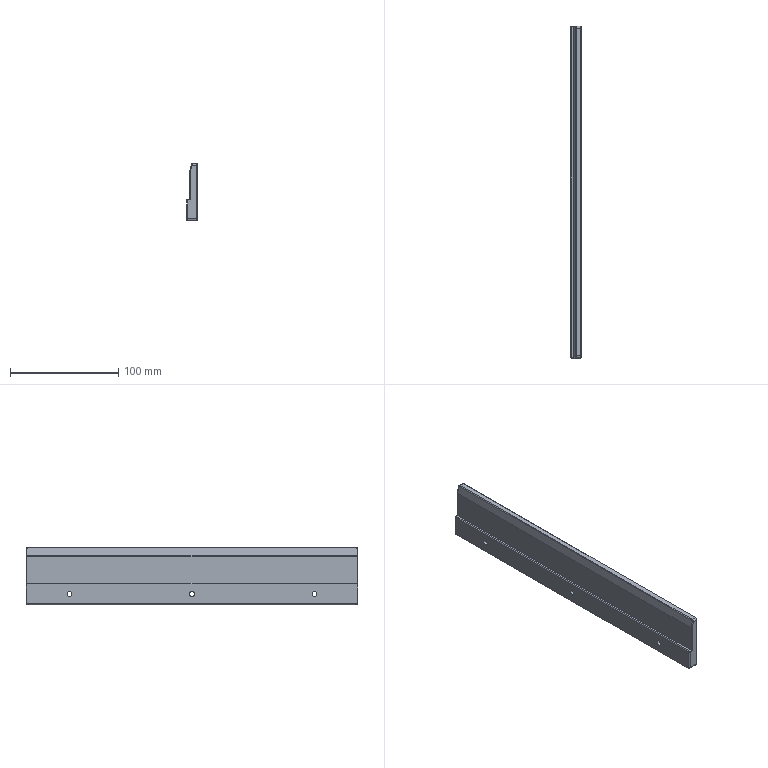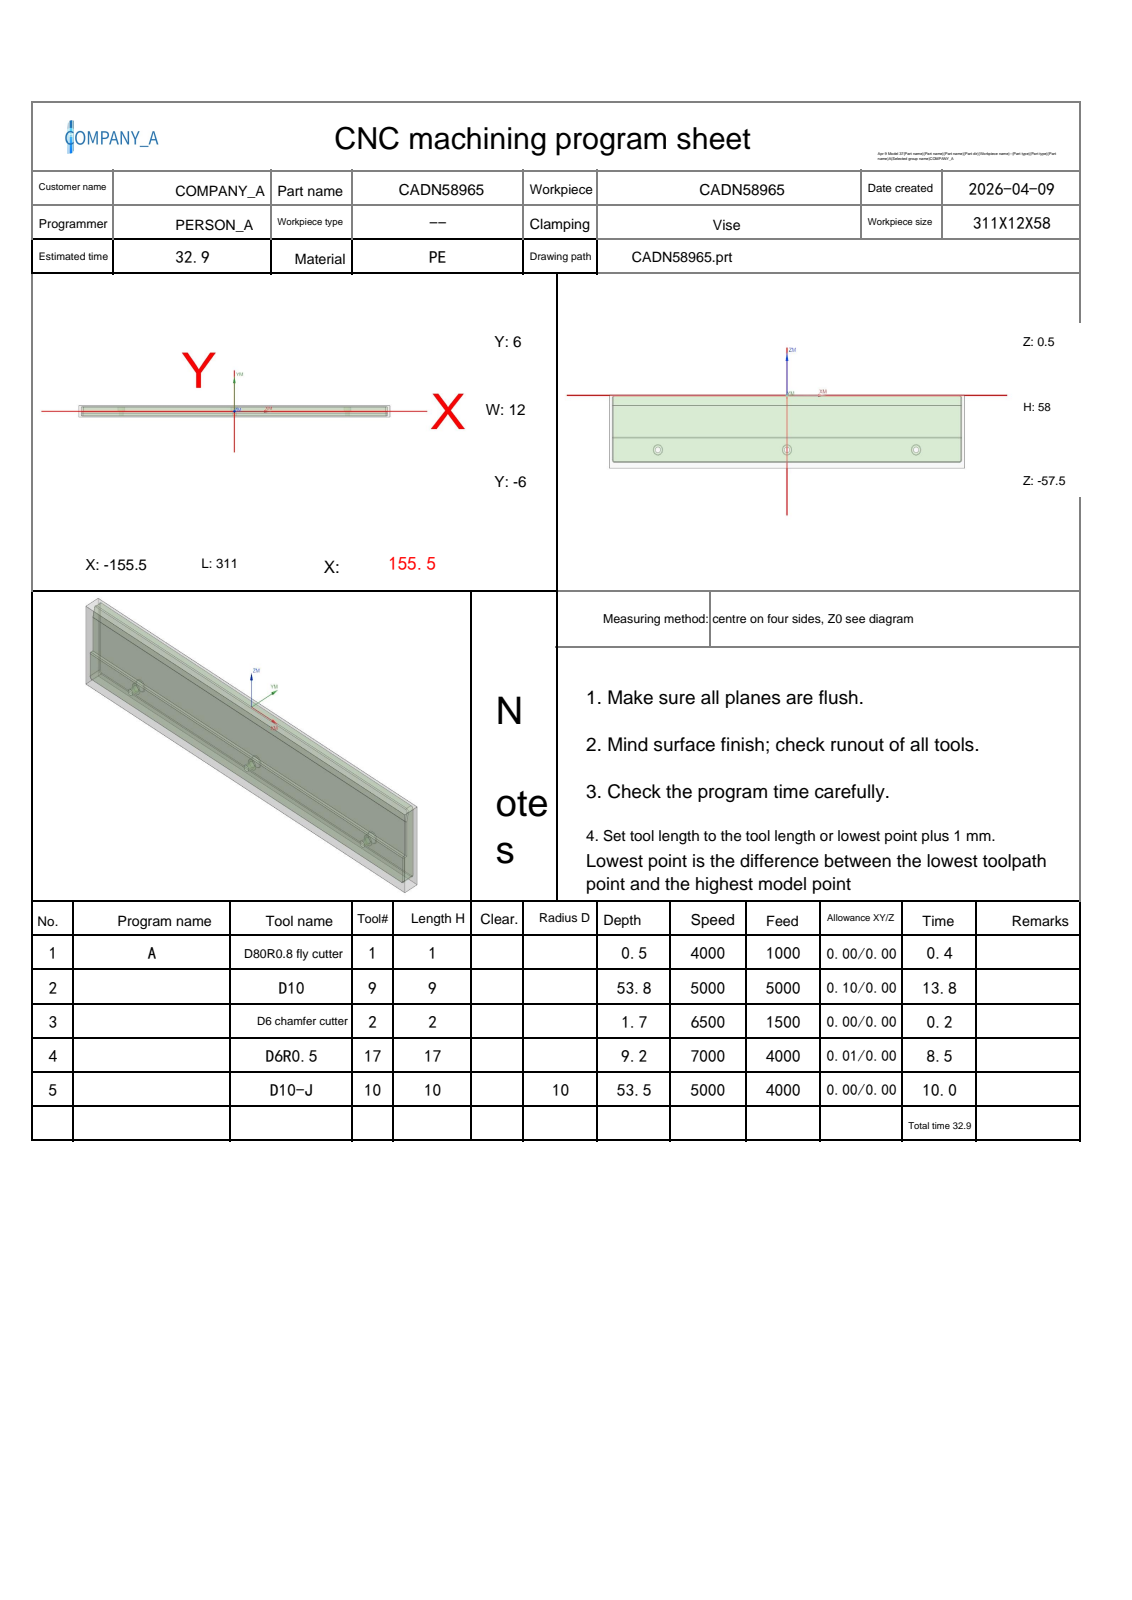NC program | NX | posted by the shop | part box 10 x 306 x 53 mm
Lines 1290 to 3098 of 3792, first 1630 of 1809 lines:
N4 T17 M06
(D6R0.5  D=6. R=0.5 H=17 ce=0.01 di=0.00)
G00 G90 G54 X148.205 Y10.104 M03 S7000
G43 H17 Z10.5
M08
Z.491
G01 Z-.009 F4000.
X148.307 Y8.501
G03 X149.804 Y7.096 I1.497 J.095
G01 X149.899 Y7.099
G02 X150.429 Y7.116 I.53 J-8.323
X151.333 Y7.067 I0.0 J-8.34
X153.721 Y4.5 I-.291 J-2.664
G01 Y.309
G02 X151.052 Y-2.343 I-2.743 J.091
G01 X149.898 Y-2.373
Y-2.418 Z-.015
Y-2.454 Z-.021
X151.047 Y-2.437
G03 X153.836 Y.283 I-.042 J2.833
G01 Y4.5
G03 X151.122 Y7.137 I-2.737 J-.102
G01 X149.9 Y7.147
Y7.179 Z-.03
Y7.2 Z-.038
G02 X150.426 Y7.214 I.526 J-9.546
X151.615 Y7.14 I0.0 J-9.56
X153.943 Y4.502 I-.331 J-2.638
G01 Y.281
G02 X151.111 Y-2.506 I-2.888 J.103
G01 X149.898 Y-2.53
Y-2.567 Z-.048
Y-2.601 Z-.058
X151.292 Y-2.578
X151.498 Y-2.553
G03 X154.046 Y.278 I-.411 J2.932
G01 Y4.5
G03 X151.508 Y7.201 I-2.811 J-.098
X150.449 Y7.253 I-1.059 J-10.844
X149.9 Y7.239 I0.0 J-10.896
G01 Y7.266 Z-.07
Y7.284 Z-.082
G02 X150.476 Y7.306 I.576 J-7.702
X151.822 Y7.188 I0.0 J-7.724
X154.147 Y4.5 I-.491 J-2.774
G01 Y.275
G02 X151.479 Y-2.618 I-3.005 J.095
X150.351 Y-2.681 I-1.128 J10.002
X149.898 Y-2.671 I0.0 J10.065
G01 Y-2.706 Z-.096
Y-2.738 Z-.111
G03 X150.415 Y-2.753 I.517 J8.965
X151.638 Y-2.67 I0.0 J8.98
X154.245 Y.271 I-.474 J3.046
G01 Y4.5
G03 X151.638 Y7.275 I-2.893 J-.105
G01 X151.292 Y7.306
X149.9 Y7.318
Y7.342 Z-.127
Y7.358 Z-.143
X151.292 Y7.34
X151.638 Y7.31
G02 X154.039 Y5.73 I-.311 J-3.086
X154.342 Y4.5 I-3.231 J-1.447
G01 Y.267
G02 X151.525 Y-2.754 I-3.126 J.091
G01 X151.292 Y-2.777
X149.898 Y-2.804
Y-2.837 Z-.16
Y-2.868 Z-.178
G03 X150.418 Y-2.884 I.52 J8.499
X151.772 Y-2.775 I0.0 J8.514
X154.437 Y.263 I-.504 J3.13
G01 Y4.5
G03 X153.915 Y6.075 I-2.8 J-.055
X151.638 Y7.346 I-2.54 J-1.874
G01 X151.292 Y7.377
X149.884 Y7.395
X149.878 Y7.435 Z-.218
X151.292 Y7.418
X151.638 Y7.385
G02 X153.639 Y6.517 I-.305 J-3.438
X154.53 Y4.519 I-1.792 J-1.998
G01 Y.258
G02 X151.871 Y-2.822 I-3.218 J.09
X150.443 Y-2.947 I-1.428 J8.105
X149.899 Y-2.929 I0.0 J8.23
G01 Y-2.96 Z-.239
Y-2.988 Z-.261
X151.19 Y-2.968
G03 X152.925 Y-2.51 I-.06 J3.748
G01 X153.022 Y-2.458
G03 X154.622 Y.253 I-1.593 J2.767
G01 Y4.5
G03 X153.714 Y6.541 I-2.829 J-.035
X151.638 Y7.429 I-2.435 J-2.823
X150.437 Y7.49 I-1.201 J-11.717
X149.9 Y7.478 I0.0 J-11.779
G01 X149.901 Y7.501 Z-.284
X149.902 Y7.524 Z-.307
G02 X150.439 Y7.537 I.536 J-11.763
X151.638 Y7.475 I0.0 J-11.775
X153.368 Y6.884 I-.506 J-4.309
X154.711 Y4.5 I-1.494 J-2.412
G01 Y.247
G02 X151.97 Y-2.928 I-3.315 J.091
X150.439 Y-3.062 I-1.531 J8.705
X149.899 Y-3.045 I0.0 J8.839
G01 Y-3.073 Z-.332
Y-3.1 Z-.357
X151.14 Y-3.088
G03 X153.017 Y-2.623 I-.04 J4.187
X154.798 Y.241 I-1.505 J2.922
G01 Y4.5
G03 X153.368 Y6.952 I-2.883 J-.039
X151.292 Y7.56 I-2.369 J-4.243
X150.427 Y7.583 I-.865 J-16.014
X149.908 Y7.575 I0.0 J-16.037
G01 Y7.601 Z-.384
Y7.628 Z-.411
G02 X150.427 Y7.637 I.519 J-16.03
X151.292 Y7.613 I0.0 J-16.038
X153.368 Y7.005 I-.334 J-4.985
X154.883 Y4.5 I-1.353 J-2.529
G01 Y.234
G02 X153.014 Y-2.7 I-3.318 J.051
X151.137 Y-3.14 I-1.915 J3.945
G01 X149.899 Y-3.151
X149.9 Y-3.176 Z-.439
Y-3.2 Z-.468
X151.292 Y-3.189
G03 X153.368 Y-2.578 I-.153 J4.354
X154.966 Y.227 I-1.743 J2.85
G01 Y4.5
G03 X153.837 Y6.765 I-2.893 J-.029
X150.946 Y7.685 I-2.911 J-4.145
G01 X149.908
Y7.715 Z-.498
Y7.745 Z-.528
G02 X150.442 Y7.757 I.534 J-11.624
X151.281 Y7.727 I0.0 J-11.637
X153.703 Y6.924 I-.375 J-5.189
X155.047 Y4.5 I-1.563 J-2.45
G01 Y.219
G02 X153.368 Y-2.656 I-3.381 J.046
X151.638 Y-3.208 I-2.168 J3.806
G01 X151.292 Y-3.236
X149.899 Y-3.245
Y-3.266 Z-.56
X149.9 Y-3.287 Z-.591
X151.292 Y-3.275
G03 X153.032 Y-2.899 I-.131 J4.811
X155.125 Y.212 I-1.331 J3.154
G01 Y4.5
G03 X154.014 Y6.765 I-2.915 J-.025
X151.638 Y7.759 I-3.257 J-4.448
X150.451 Y7.821 I-1.187 J-11.365
X149.921 Y7.808 I0.0 J-11.427
G01 X149.923 Y7.842 Z-.624
X149.925 Y7.875 Z-.658
G02 X150.37 Y7.882 I.446 J-13.896
X151.638 Y7.824 I0.0 J-13.903
X153.714 Y7.024 I-.919 J-5.48
G01 X154.06 Y6.792
G02 X155.2 Y4.5 I-1.776 J-2.312
G01 Y.203
G02 X153.368 Y-2.798 I-3.435 J.037
X151.638 Y-3.293 I-2.048 J3.893
X150.427 Y-3.333 I-1.212 J18.322
X149.902 Y-3.325 I0.0 J18.362
G01 X149.903 Y-3.343 Z-.692
Y-3.36 Z-.727
X151.292 Y-3.352
G03 X153.3 Y-2.899 I-.031 J4.805
X155.272 Y.195 I-1.495 J3.128
G01 Y4.502
G03 X153.98 Y6.902 I-2.876 J0.0
G01 X153.714 Y7.078
G03 X151.638 Y7.89 I-2.966 J-4.523
X150.362 Y7.951 I-1.277 J-13.299
X149.928 Y7.944 I0.0 J-13.361
G01 X149.93 Y7.979 Z-.762
X149.932 Y8.015 Z-.797
G02 X150.353 Y8.022 I.422 J-12.842
X151.638 Y7.957 I0.0 J-12.849
X153.75 Y7.11 I-.89 J-5.274
X155.063 Y5.73 I-1.5 J-2.741
X155.341 Y4.516 I-2.509 J-1.213
G01 Y.186
G02 X152.676 Y-3.192 I-3.558 J.067
X151.292 Y-3.384 I-1.455 J5.416
G01 X149.905 Y-3.39
Y-3.403 Z-.833
X149.906 Y-3.415 Z-.868
X151.292 Y-3.409
G03 X152.676 Y-3.242 I-.052 J6.248
X153.842 Y-2.713 I-1.122 J4.023
X155.404 Y.177 I-1.893 J2.89
G01 Y4.505
G03 X154.688 Y6.402 I-2.871 J0.0
X153.836 Y7.11 I-2.68 J-2.36
X151.638 Y8.024 I-3.127 J-4.418
X150.347 Y8.092 I-1.291 J-12.294
X149.935 Y8.085 I0.0 J-12.362
G01 X149.937 Y8.121 Z-.903
X149.938 Y8.156 Z-.939
X150.918 Y8.15
G02 X152.911 Y7.692 I-.027 J-4.685
X154.406 Y6.748 I-3.268 J-6.835
X155.463 Y4.5 I-1.912 J-2.271
G01 Y.168
G02 X153.368 Y-3.037 I-3.547 J.031
X151.638 Y-3.423 I-1.837 J4.166
X150.169 Y-3.435 I-1.469 J84.542
G01 X149.908
Y-3.444 Z-.974
Y-3.453 Z-1.009
X151.638 Y-3.442
X151.65
G03 X153.368 Y-3.087 I0.0 J4.335
X155.517 Y.159 I-1.416 J3.272
G01 Y4.5
G03 X154.406 Y6.796 I-2.973 J-.021
X153.022 Y7.698 I-5.152 J-6.395
X150.946 Y8.22 I-2.136 J-4.103
G01 X149.942 Y8.227
X149.944 Y8.262 Z-1.045
X149.945 Y8.297 Z-1.08
X150.946 Y8.291
G02 X153.022 Y7.758 I-.07 J-4.583
X154.537 Y6.731 I-3.987 J-7.508
X155.568 Y4.504 I-1.891 J-2.227
G01 Y.15
G02 X153.817 Y-2.903 I-3.578 J.024
X151.896 Y-3.455 I-2.015 J3.393
G01 X151.638 Y-3.461
X149.908 Y-3.47
Y-3.488 Z-1.151
X151.984 Y-3.476
G03 X153.368 Y-3.17 I-.157 J3.988
G01 X153.714 Y-3.006
G03 X155.615 Y.141 I-1.693 J3.17
G01 Y4.501
G03 X154.622 Y6.699 I-2.93 J0.0
X153.022 Y7.818 I-5.769 J-6.545
X150.946 Y8.362 I-2.151 J-3.979
G01 X149.949 Y8.368
X149.951 Y8.404 Z-1.186
X149.952 Y8.439 Z-1.222
X150.946 Y8.432
G02 X153.022 Y7.875 I-.07 J-4.409
X154.752 Y6.627 I-4.466 J-8.012
X155.658 Y4.5 I-2.091 J-2.148
G01 Y.132
G02 X153.4 Y-3.199 I-3.619 J.023
X151.867 Y-3.5 I-1.545 J3.809
G01 X149.91 Y-3.506
X149.914 Y-3.523 Z-1.292
X151.984 Y-3.519
G03 X153.022 Y-3.365 I-.081 J4.102
X155.444 Y-1.203 I-.978 J3.533
X155.699 Y.123 I-3.847 J1.427
G01 Y4.5
X155.647 Y5.039
G03 X154.752 Y6.67 I-2.959 J-.563
X153.022 Y7.933 I-6.858 J-7.578
X150.946 Y8.503 I-2.145 J-3.749
G01 X150.029 Y8.508
X150.187 Y8.544 Z-1.328
X150.346 Y8.577 Z-1.363
G02 X150.611 Y8.582 I.265 J-7.205
X151.258 Y8.553 I0.0 J-7.21
X153.165 Y7.91 I-.387 J-4.298
X154.681 Y6.765 I-5.864 J-9.342
G01 X154.752 Y6.706
G02 X155.686 Y5.039 I-2.016 J-2.224
G01 X155.736 Y4.5
Y.114
G02 X155.676 Y-.484 I-4.918 J.197
X153.214 Y-3.334 I-3.554 J.582
G01 X153.139 Y-3.358
G02 X151.983 Y-3.538 I-1.162 J3.653
G01 X149.918 Y-3.541
X149.922 Y-3.559 Z-1.434
X151.984 Y-3.557
X152.04
G03 X155.098 Y-2. I0.0 J3.781
X155.771 Y.105 I-3.13 J2.161
G01 Y4.5
G03 X154.752 Y6.739 I-3.003 J-.015
G01 X154.721 Y6.765
G03 X153.022 Y8.048 I-7.837 J-8.607
X150.906 Y8.645 I-2.143 J-3.547
G01 X151.071 Y8.654 Z-1.446
X151.237 Y8.652 Z-1.458
X151.403 Y8.646 Z-1.47
X151.569 Y8.637 Z-1.482
X151.733 Y8.618 Z-1.494
X151.893 Y8.586 Z-1.506
G02 X152.956 Y8.145 I-.944 J-3.783
X154.406 Y7.071 I-5.053 J-8.337
X155.098 Y6.424 I-3.857 J-4.819
X155.804 Y4.5 I-2.316 J-1.941
G01 Y.096
G02 X154.241 Y-2.899 I-3.698 J.025
X152.044 Y-3.577 I-2.197 J3.22
G01 X151.984 Y-3.576
X149.926 Y-3.577
X149.941 Y-3.596 Z-1.583
X151.984
X152.056 Y-3.597
G03 X153.703 Y-3.244 I0.0 J4.018
X155.836 Y.086 I-1.561 J3.348
G01 Y4.502
G03 X154.893 Y6.674 I-2.975 J0.0
X153.368 Y7.941 I-11.484 J-12.272
X152.464 Y8.462 I-3.017 J-4.194
G01 X152.586 Y8.431 Z-1.61
X152.706 Y8.397 Z-1.637
X152.818 Y8.348 Z-1.665
G02 X153.368 Y7.998 I-2.023 J-3.785
X154.941 Y6.658 I-11.701 J-15.325
X155.866 Y4.503 I-2.045 J-2.155
G01 Y.076
G02 X155.643 Y-1.173 I-3.923 J.057
X153.368 Y-3.411 I-3.466 J1.247
X152.064 Y-3.617 I-1.304 J4.028
G01 X151.984
X149.935
X149.931 Y-3.638 Z-1.75
X151.984
X152.33 Y-3.63
G03 X155.537 Y-1.518 I-.137 J3.698
X155.895 Y.066 I-3.548 J1.634
G01 Y4.503
G03 X155.013 Y6.612 I-2.963 J0.0
X154.089 Y7.455 I-11.248 J-11.398
X153.082 Y8.255 I-5.983 J-6.492
G01 X153.184 Y8.221 Z-1.794
X153.278 Y8.175 Z-1.838
G02 X154.131 Y7.455 I-5.786 J-7.721
X154.882 Y6.765 I-7.706 J-9.141
G01 X154.985 Y6.668
G02 X155.921 Y4.501 I-2.041 J-2.167
G01 Y.055
G02 X152.33 Y-3.652 I-3.714 J.004
G01 X151.984 Y-3.66
X150.
X150.106 Y-3.683 Z-1.931
X151.984
X152.33 Y-3.676
G03 X154.891 Y-2.553 I-.104 J3.718
X155.944 Y.043 I-2.739 J2.623
G01 Y4.505
G03 X155.071 Y6.606 I-2.963 J0.0
X153.425 Y8.116 I-19.463 J-19.56
G01 X153.532 Y8.074 Z-2.026
X153.714 Y7.917
X154.752 Y6.944
X155.061 Y6.644
G02 X155.965 Y4.503 I-2.084 J-2.141
G01 Y.032
G02 X154.406 Y-3.009 I-3.781 J.018
X152.33 Y-3.7 I-2.174 J3.065
G01 X150.946 Y-3.707
X150.6
X151.072 Y-3.731 Z-2.122
X152.33 Y-3.725
G03 X155.981 Y.016 I-.092 J3.741
G01 Y.02
Y4.5
G03 X155.098 Y6.627 I-3.013 J-.004
X153.633 Y8.024 I-51.022 J-52.063
G01 X153.721 Y7.976 Z-2.216
G02 X155.098 Y6.638 I-135.624 J-140.96
X155.994 Y4.5 I-2.108 J-2.14
G01 Y.008
G02 X153.347 Y-3.589 I-3.775 J.005
X152.212 Y-3.75 I-1.153 J4.054
G01 X151.103 Y-3.754
X151.134 Y-3.778 Z-2.311
X152.216 Y-3.774
G03 X153.368 Y-3.606 I-.017 J4.157
X156.003 Y-.003 I-1.152 J3.607
G01 Y4.5
G03 X155.098 Y6.645 I-3.03 J-.015
G01 X154.976 Y6.765
X153.76 Y7.959
X153.795 Y7.938 Z-2.405
X154.06 Y7.679
X155.12 Y6.631
G02 X156.008 Y4.502 I-2.106 J-2.129
G01 Y-.015
G02 X153.368 Y-3.63 I-3.797 J.002
X152.217 Y-3.798 I-1.165 J3.953
G01 X151.133 Y-3.802
X151.164 Y-3.825 Z-2.5
X151.292
X152.33 Y-3.822
G03 X156.008 Y-.138 I-.098 J3.775
G01 X156.01 Y-.015
Y4.511
G03 X155.098 Y6.659 I-3.012 J-.011
G01 X153.831 Y7.918
G00 Z10.5
X-146.979 Y-5.373
Z.491
G01 Z-.009
Y-5.372
G03 X-149.898 Y-2.373 I-3. J0.0
G01 X-151.056 Y-2.342
G02 X-153.721 Y.284 I.073 J2.74
G01 Y4.5
G02 X-151.333 Y7.067 I2.678 J-.097
X-150.429 Y7.116 I.904 J-8.294
X-149.899 Y7.099 I0.0 J-8.343
G01 X-149.9 Y7.132 Z-.015
Y7.147 Z-.021
X-151.122 Y7.137
G03 X-153.836 Y4.5 I.024 J-2.739
G01 Y.283
G03 X-151.048 Y-2.437 I2.83 J.112
G01 X-149.898 Y-2.454
Y-2.495 Z-.03
Y-2.53 Z-.038
X-151.292 Y-2.503
G02 X-153.943 Y.281 I.221 J2.864
G01 Y4.501
G02 X-151.638 Y7.137 I2.66 J0.0
X-150.451 Y7.217 I1.188 J-8.811
X-149.9 Y7.2 I0.0 J-8.891
G01 Y7.223 Z-.048
Y7.239 Z-.058
G03 X-150.45 Y7.253 I-.549 J-10.88
X-151.508 Y7.201 I0.0 J-10.894
X-154.046 Y4.5 I.273 J-2.8
G01 Y.278
G03 X-151.498 Y-2.553 I2.959 J.1
G01 X-151.292 Y-2.578
X-149.898 Y-2.601
Y-2.638 Z-.07
Y-2.671 Z-.082
G02 X-150.351 Y-2.681 I-.453 J10.055
X-151.479 Y-2.618 I0.0 J10.065
X-154.147 Y.275 I.337 J2.987
G01 Y4.5
G02 X-151.638 Y7.23 I2.857 J-.107
X-150.407 Y7.295 I1.231 J-11.584
X-149.9 Y7.284 I0.0 J-11.649
G01 Y7.305 Z-.096
Y7.318 Z-.111
X-151.292 Y7.306
X-151.638 Y7.275
G03 X-154.245 Y4.5 I.286 J-2.881
G01 Y.271
G03 X-151.638 Y-2.67 I3.081 J.105
X-150.415 Y-2.753 I1.223 J8.896
X-149.898 Y-2.738 I0.0 J8.98
G01 Y-2.772 Z-.127
Y-2.804 Z-.143
X-151.292 Y-2.777
X-151.525 Y-2.754
G02 X-154.342 Y.267 I.309 J3.112
G01 Y4.5
G02 X-153.022 Y6.823 I2.806 J-.058
G01 X-152.789 Y6.947
G02 X-151.262 Y7.34 I1.57 J-2.938
G01 X-149.9 Y7.358
X-149.884 Y7.395 Z-.178
X-151.267 Y7.377
G03 X-152.812 Y7. I.046 J-3.545
G01 X-153.022 Y6.895
G03 X-154.437 Y4.5 I1.427 J-2.458
G01 Y.263
G03 X-151.772 Y-2.775 I3.169 J.092
X-150.418 Y-2.884 I1.354 J8.406
X-149.898 Y-2.868 I0.0 J8.514
G01 X-149.899 Y-2.899 Z-.198
Y-2.929 Z-.218
G02 X-150.443 Y-2.947 I-.545 J8.212
X-151.871 Y-2.822 I0.0 J8.23
X-154.53 Y.258 I.558 J3.17
G01 Y4.5
G02 X-153.026 Y6.959 I2.841 J-.048
X-151.231 Y7.419 I1.84 J-3.454
G01 X-149.878 Y7.435
X-149.9 Y7.478 Z-.261
G03 X-150.437 Y7.49 I-.538 J-11.767
X-151.638 Y7.429 I0.0 J-11.779
X-153.368 Y6.815 I.431 J-3.958
X-154.622 Y4.5 I1.58 J-2.352
G01 Y.23
G03 X-154.406 Y-.856 I2.843 J0.0
X-151.691 Y-2.919 I3.121 J1.289
X-150.372 Y-2.999 I1.319 J10.898
X-149.899 Y-2.988 I0.0 J10.977
G01 Y-3.018 Z-.284
Y-3.045 Z-.307
G02 X-150.439 Y-3.062 I-.54 J8.822
X-151.97 Y-2.928 I0.0 J8.839
X-154.711 Y.247 I.574 J3.266
G01 Y4.501
G02 X-153.31 Y6.918 I2.785 J0.0
X-151.292 Y7.509 I2.243 J-3.914
X-150.424 Y7.533 I.868 J-16.089
X-149.902 Y7.524 I0.0 J-16.112
G01 X-149.905 Y7.55 Z-.332
X-149.908 Y7.575 Z-.357
X-150.946
G03 X-153.368 Y6.952 I.003 J-5.034
X-154.798 Y4.5 I1.453 J-2.491
G01 Y.241
G03 X-154.06 Y-1.781 I3.311 J.063
X-151.638 Y-3.05 I2.816 J2.428
G01 X-151.292 Y-3.086
X-149.899 Y-3.1
Y-3.126 Z-.384
Y-3.151 Z-.411
X-151.191 Y-3.141
G02 X-153.752 Y-2.208 I.03 J4.066
X-154.883 Y.234 I2.163 J2.485
G01 Y4.5
G02 X-153.368 Y7.005 I2.868 J-.024
X-150.946 Y7.628 I2.447 J-4.492
G01 X-149.908
Y7.657 Z-.439
Y7.685 Z-.468
X-150.946
G03 X-153.837 Y6.765 I.026 J-5.081
X-154.966 Y4.5 I1.764 J-2.294
G01 Y.227
G03 X-153.368 Y-2.578 I3.34 J.045
X-151.292 Y-3.189 I2.228 J3.743
G01 X-149.9 Y-3.2
X-149.899 Y-3.223 Z-.498
Y-3.245 Z-.528
X-151.292 Y-3.236
X-151.638 Y-3.208
G02 X-153.368 Y-2.656 I.438 J4.358
X-155.047 Y.219 I1.702 J2.921
G01 Y4.511
G02 X-153.814 Y6.844 I2.826 J0.0
X-150.946 Y7.745 I2.918 J-4.273
G01 X-149.908
X-149.915 Y7.777 Z-.56
X-149.921 Y7.808 Z-.591
X-150.946
X-151.04 Y7.805
G03 X-154.06 Y6.725 I.166 J-5.225
X-155.125 Y4.5 I1.836 J-2.246
G01 Y.212
G03 X-153.032 Y-2.899 I3.424 J.044
X-151.292 Y-3.275 I1.871 J4.434
G01 X-149.9 Y-3.287
X-149.901 Y-3.307 Z-.624
X-149.902 Y-3.325 Z-.658
G02 X-150.372 Y-3.33 I-.47 J21.278
X-151.638 Y-3.293 I0.0 J21.283
X-153.689 Y-2.602 I.283 J4.232
X-155.2 Y.202 I1.847 J2.804
G01 Y4.5
G02 X-154.06 Y6.792 I2.916 J-.021
G01 X-153.807 Y6.962
G02 X-151.638 Y7.824 I3.078 J-4.586
X-150.361 Y7.881 I1.278 J-14.183
X-149.925 Y7.875 I0.0 J-14.24
G01 X-149.926 Y7.909 Z-.692
X-149.928 Y7.944 Z-.727
G03 X-150.351 Y7.95 I-.423 J-13.678
X-151.638 Y7.89 I0.0 J-13.685
X-153.714 Y7.078 I.889 J-5.332
G01 X-154.06 Y6.849
G03 X-155.272 Y4.5 I1.705 J-2.367
G01 Y.195
G03 X-153.3 Y-2.899 I3.467 J.035
X-151.292 Y-3.352 I2.039 J4.352
G01 X-149.904 Y-3.36
Y-3.375 Z-.762
X-149.905 Y-3.39 Z-.797
X-151.292 Y-3.384
G02 X-152.676 Y-3.192 I.072 J5.61
X-155.341 Y.186 I.894 J3.445
G01 Y4.501
G02 X-154.16 Y6.835 I2.897 J0.0
X-152.676 Y7.672 I4.204 J-5.718
X-150.946 Y8.01 I1.738 J-4.301
G01 X-149.932 Y8.014
X-149.933 Y8.05 Z-.833
X-149.935 Y8.085 Z-.868
X-150.999 Y8.079
G03 X-152.67 Y7.738 I.024 J-4.38
X-154.321 Y6.765 I2.748 J-6.548
X-155.404 Y4.5 I1.867 J-2.284
G01 Y.176
G03 X-154.946 Y-1.532 I3.413 J0.0
X-153.022 Y-3.128 I3.12 J1.803
X-151.638 Y-3.395 I1.573 J4.426
X-150.381 Y-3.418 I1.258 J35.315
X-149.908 Y-3.415 I0.0 J35.337
G01 Y-3.425 Z-.903
Y-3.435 Z-.939
X-150.171
G02 X-151.638 Y-3.423 I0.0 J84.221
X-153.368 Y-3.037 I.107 J4.551
X-155.463 Y.168 I1.452 J3.236
G01 Y4.5
G02 X-154.406 Y6.748 I2.969 J-.022
X-152.91 Y7.693 I4.761 J-5.889
X-150.927 Y8.149 I2.014 J-4.216
G01 X-149.939 Y8.156
X-149.94 Y8.191 Z-.974
X-149.942 Y8.226 Z-1.009
X-150.946 Y8.219
G03 X-153.022 Y7.698 I.056 J-4.617
X-154.406 Y6.796 I3.766 J-7.294
X-155.517 Y4.5 I1.863 J-2.318
G01 Y.159
G03 X-153.737 Y-2.899 I3.553 J.022
X-151.67 Y-3.442 I2.067 J3.661
G01 X-151.638
X-149.909 Y-3.453
X-149.913 Y-3.47 Z-1.08
X-151.638 Y-3.461
X-151.896 Y-3.455
G02 X-153.817 Y-2.903 I.094 J3.945
X-155.568 Y.15 I1.827 J3.076
G01 Y4.503
G02 X-154.536 Y6.732 I2.923 J0.0
X-153.022 Y7.758 I5.499 J-6.479
X-150.946 Y8.29 I2.143 J-4.047
G01 X-149.946 Y8.297
X-149.947 Y8.333 Z-1.116
X-149.949 Y8.367 Z-1.151
X-150.946 Y8.361
G03 X-153.022 Y7.818 I.073 J-4.522
X-154.623 Y6.698 I4.167 J-7.661
X-155.615 Y4.501 I1.937 J-2.197
G01 Y.141
G03 X-154.379 Y-2.553 I3.629 J.034
X-151.875 Y-3.477 I2.527 J2.995
G01 X-149.917 Y-3.488
X-149.921 Y-3.506 Z-1.222
X-151.917 Y-3.5
G02 X-153.931 Y-2.929 I.011 J3.88
X-155.658 Y.132 I1.887 J3.082
G01 Y4.5
G02 X-154.752 Y6.627 I3.008 J-.025
X-153.022 Y7.875 I6.194 J-6.761
X-150.946 Y8.431 I2.144 J-3.853
G01 X-149.952 Y8.438
X-150.027 Y8.507 Z-1.292
X-150.946 Y8.502
G03 X-153.022 Y7.933 I.067 J-4.317
X-154.752 Y6.67 I5.125 J-8.836
X-155.699 Y4.5 I2.094 J-2.205
G01 Y.123
G03 X-155.455 Y-1.173 I4.106 J.102
X-154.055 Y-2.899 I3.413 J1.339
X-151.984 Y-3.519 I2.125 J3.324
G01 X-149.925 Y-3.523
X-149.929 Y-3.541 Z-1.363
X-151.984 Y-3.538
X-151.986
G02 X-154.56 Y-2.553 I0.0 J3.858
X-155.607 Y-.828 I2.495 J2.693
X-155.736 Y.114 I4.788 J1.139
G01 Y4.5
G02 X-154.752 Y6.706 I3.035 J-.032
X-153.022 Y7.991 I7.506 J-8.297
X-150.946 Y8.572 I2.14 J-3.643
G01 X-150.34 Y8.575
X-150.478 Y8.593 Z-1.381
X-150.615 Y8.61 Z-1.398
X-150.753 Y8.626 Z-1.416
X-150.891 Y8.641 Z-1.434
X-150.9
G03 X-153.022 Y8.048 I0.0 J-4.094
X-154.406 Y7.035 I4.969 J-8.238
G01 X-154.721 Y6.765
X-154.752 Y6.739
G03 X-155.771 Y4.5 I1.986 J-2.255
G01 Y.105
G03 X-155.098 Y-2. I3.803 J.056
X-152.04 Y-3.557 I3.058 J2.224
G01 X-151.984
X-149.933 Y-3.559
X-149.938 Y-3.577 Z-1.506
X-151.984 Y-3.576
X-152.236 Y-3.567
G02 X-155.098 Y-2.06 I.136 J3.729
X-155.804 Y.096 I3.065 J2.197
G01 Y4.5
G02 X-154.752 Y6.773 I3.017 J-.017
G01 X-154.406 Y7.071
X-154.365 Y7.11
G02 X-153.022 Y8.107 I6.848 J-7.817
X-151.895 Y8.585 I2.119 J-3.428
G01 X-152.041 Y8.567 Z-1.525
X-152.185 Y8.54 Z-1.545
X-152.327 Y8.506 Z-1.564
X-152.464 Y8.462 Z-1.583
G03 X-153.368 Y7.941 I2.114 J-4.719
X-154.892 Y6.675 I9.957 J-13.537
X-155.836 Y4.501 I2.034 J-2.174
G01 Y.086
G03 X-154.752 Y-2.512 I3.705 J.02
X-152.293 Y-3.589 I2.644 J2.693
G01 X-151.984 Y-3.596
X-149.943
X-149.936 Y-3.617 Z-1.665
X-151.984
X-152.241 Y-3.61
G02 X-154.752 Y-2.564 I.094 J3.762
X-155.79 Y-.66 I2.652 J2.68
X-155.866 Y.076 I6.088 J1.002
G01 Y4.501
G02 X-154.976 Y6.619 I2.965 J0.0
G01 X-154.827 Y6.765
G02 X-153.368 Y7.998 I13.147 J-14.078
X-152.818 Y8.348 I2.574 J-3.439
G01 X-152.954 Y8.308 Z-1.707
X-153.082 Y8.255 Z-1.75
G03 X-153.793 Y7.713 I4.151 J-6.171
G01 X-154.06 Y7.482
G03 X-155.005 Y6.621 I11.734 J-13.821
X-155.895 Y4.505 I2.07 J-2.116
G01 Y.066
G03 X-155.849 Y-.466 I4.881 J.155
X-152.288 Y-3.631 I3.647 J.518
G01 X-151.984 Y-3.638
X-149.932
X-150.005 Y-3.66 Z-1.838
X-151.984
X-152.33 Y-3.652
G02 X-155.917 Y.041 I.117 J3.702
G01 X-155.921 Y.055
Y4.505
G02 X-155.025 Y6.63 I2.969 J0.0
X-153.368 Y8.11 I17.675 J-18.121
G01 X-153.278 Y8.175
X-153.425 Y8.116 Z-1.931
G03 X-154.408 Y7.241 I13.777 J-16.453
G01 X-155.011 Y6.669
G03 X-155.944 Y4.5 I2.055 J-2.169
G01 Y.043
G03 X-155.833 Y-.828 I3.686 J.028
X-152.33 Y-3.676 I3.599 J.848
G01 X-151.984 Y-3.683
X-150.254
X-150.6 Y-3.707 Z-2.026
G02 X-151.292 Y-3.712 I-.692 J46.254
X-152.33 Y-3.7 I0.0 J46.259
X-155.96 Y-.001 I.093 J3.721
G01 X-155.965 Y.032
Y4.5
G02 X-155.098 Y6.609 I3.014 J-.006
X-153.531 Y8.074 I28.571 J-28.991
G01 X-153.633 Y8.024 Z-2.122
G03 X-155.098 Y6.627 I50.352 J-54.286
X-155.981 Y4.5 I2.142 J-2.136
G01 Y.02
G02 X-155.969 Y-.2 I-178.686 J-10.13
G03 X-152.26 Y-3.725 I3.726 J.207
G01 X-151.067 Y-3.731
X-151.127 Y-3.754 Z-2.216
X-152.33 Y-3.749
G02 X-155.99 Y-.005 I.086 J3.744
G01 Y-.001
X-155.994 Y.008
Y4.5
G02 X-155.098 Y6.64 I3.03 J-.011
X-153.721 Y7.976 I635.69 J-653.794
G01 X-153.76 Y7.959 Z-2.311
X-155.186 Y6.562
G03 X-156.003 Y4.5 I2.236 J-2.079
G01 Y-.003
Y-.01
G03 X-152.33 Y-3.773 I3.765 J0.0
G01 X-151.125 Y-3.778
X-151.154 Y-3.802 Z-2.405
X-152.33 Y-3.798
G02 X-156.008 Y-.025 I.095 J3.772
G01 Y-.015
Y4.502
G02 X-155.118 Y6.635 I2.998 J0.0
G01 X-153.938 Y7.8
X-153.795 Y7.938
X-153.832 Y7.918 Z-2.5
X-153.95 Y7.8
X-155.098 Y6.659
G03 X-156.01 Y4.518 I2.1 J-2.158
G01 Y-.028
X-156.008 Y-.138
G03 X-152.33 Y-3.822 I3.776 J.091
G01 X-151.152 Y-3.825
G00 Z10.5
G00 G90 X156.74 Y4.398 M03 S7000
Z10.5
Z.489
G01 Z-.011 F4000.
G03 X153.74 Y1.398 I0.0 J-3.
G02 X153.769 Y.88 I-4.67 J-.518
X153.602 Y-.363 I-4.699 J0.0
X151. Y-2.387 I-2.655 J.728
G01 X-151.
G02 X-153.725 Y.365 I.07 J2.794
G01 X-153.74 Y1.398
X-153.808 Y1.397 Z-.018
X-153.862 Y1.396 Z-.025
X-153.811 Y.181
G03 X-151.044 Y-2.473 I2.767 J.116
G01 X151.038
G03 X153.819 Y.208 I0.0 J2.782
G01 X153.862 Y1.396
X153.92 Y1.395 Z-.034
X153.97 Y1.394 Z-.043
G02 X153.981 Y1.02 I-6.446 J-.374
X153.85 Y-.273 I-6.456 J0.0
X151.063 Y-2.548 I-2.787 J.57
G01 X-151.045
G02 X-153.936 Y.279 I0.0 J2.892
G01 X-153.961 Y1.377
X-153.97 Y1.394
X-154.024 Y1.395 Z-.053
X-154.072 Z-.064
X-154.064 Y.363
G03 X-151.056 Y-2.619 I3.008 J.025
G01 X151.076
G03 X153.93 Y-.448 I0.0 J2.961
X154.104 Y.839 I-4.653 J1.288
X154.072 Y1.395 I-4.828 J0.0
G01 X154.124 Y1.393 Z-.077
X154.172 Y1.392 Z-.089
X154.103 Y-.271
G02 X151.068 Y-2.689 I-3.035 J.696
G01 X151. Y-2.688
X-151.
X-151.068 Y-2.689
G02 X-154.103 Y-.271 I0.0 J3.114
G01 X-154.172 Y1.392
X-154.223 Y1.39 Z-.104
X-154.27 Y1.388 Z-.118
G03 X-154.283 Y.97 I6.765 J-.418
X-154.052 Y-.786 I6.778 J0.0
X-151.074 Y-2.756 I2.978 J1.265
G01 X-151. Y-2.755
X151.
X151.074 Y-2.756
G03 X154.052 Y-.786 I0.0 J3.236
X154.283 Y.97 I-6.547 J1.756
X154.27 Y1.388 I-6.778 J0.0
G01 X154.32 Y1.386 Z-.135
X154.367 Y1.385 Z-.151
G02 X154.39 Y.865 I-5.688 J-.52
X154.092 Y-.957 I-5.712 J0.0
X151.071 Y-2.821 I-3.021 J1.517
G01 X151.
X-151.
X-151.071
G02 X-154.092 Y-.957 I0.0 J3.381
X-154.39 Y.865 I5.414 J1.822
X-154.367 Y1.385 I5.712 J0.0
G01 X-154.415 Y1.379 Z-.17
X-154.461 Y1.373 Z-.188
X-154.456 Y.212
G03 X-153.755 Y-1.654 I2.865 J.012
X-151.057 Y-2.884 I2.698 J2.342
G01 X-151.
X151.
G03 X152.533 Y-2.559 I-.055 J4.037
X154.453 Y.325 I-1.245 J2.91
G01 X154.461 Y1.373
X154.509 Y1.37 Z-.208
X154.554 Y1.368 Z-.228
G02 X154.572 Y.86 I-7.148 J-.508
X154.495 Y-.186 I-7.166 J0.0
X152.429 Y-2.686 I-3.099 J.457
X151. Y-2.945 I-1.53 J4.382
G01 X-151.
X-151.037
G02 X-153.705 Y-1.845 I0.0 J3.787
X-154.545 Y.072 I2.319 J2.159
G01 X-154.552 Y.415
X-154.554 Y1.368
X-154.6 Y1.365 Z-.25
X-154.645 Y1.363 Z-.272
X-154.64 Y.259
G03 X-153.327 Y-2.275 I3.127 J.013
X-151.047 Y-3.004 I2.28 J3.201
G01 X-151. Y-3.003
X151.
G03 X152.616 Y-2.684 I-.045 J4.477
X154.64 Y.291 I-1.194 J2.988
G01 X154.645 Y1.363
X154.69 Y1.36 Z-.296
X154.734 Y1.358 Z-.32
X154.732 Y.307
G02 X152.893 Y-2.628 I-3.266 J.004
X151.014 Y-3.06 I-1.878 J3.87
G01 X151.
X-151.
X-151.023
G02 X-152.988 Y-2.578 I0.0 J4.253
X-154.732 Y.294 I1.498 J2.876
G01 X-154.734 Y1.358
X-154.778 Y1.356 Z-.345
X-154.82 Y1.355 Z-.371
X-154.816 Y.27
G03 X-152.895 Y-2.701 I3.278 J.013
X-151. Y-3.113 I1.902 J4.183
G01 X151.
G03 X152.907 Y-2.695 I-.008 J4.595
X154.813 Y.252 I-1.361 J2.97
G01 X154.82 Y1.355
X154.864 Y1.351 Z-.398
X154.905 Y1.348 Z-.425
X154.904 Y.278
G02 X152.951 Y-2.746 I-3.325 J.004
X151.018 Y-3.164 I-1.933 J4.266
G01 X151.
X-151.
X-151.018
G02 X-152.951 Y-2.746 I0.0 J4.683
X-154.904 Y.278 I1.373 J3.028
G01 X-154.905 Y1.348
X-154.947 Y1.345 Z-.454
X-154.987 Y1.342 Z-.483
X-154.983 Y1.326
Y.248
G03 X-153.203 Y-2.69 I3.314 J0.0
X-151.075 Y-3.212 I2.128 J4.077
G01 X-151.
X151.
X151.075
G03 X153.203 Y-2.69 I0.0 J4.599
X154.983 Y.248 I-1.534 J2.938
G01 Y1.326
X154.987 Y1.342
X155.028 Y1.338 Z-.514
X155.067 Y1.335 Z-.544
X155.065 Y1.32
Y.266
G02 X152.938 Y-2.892 I-3.408 J0.0
X151.071 Y-3.256 I-1.867 J4.603
G01 X151.
X-151.
X-151.071
G02 X-152.938 Y-2.892 I0.0 J4.967
X-155.065 Y.266 I1.281 J3.158
G01 Y1.32
X-155.067 Y1.335
X-155.106 Y1.328 Z-.576
X-155.144 Y1.322 Z-.608
X-155.14 Y.234
G03 X-152.991 Y-2.931 I3.424 J.013
X-151.092 Y-3.298 I1.899 J4.733
G01 X-151. Y-3.297
X151.
X151.092 Y-3.298
G03 X152.991 Y-2.931 I0.0 J5.099
X155.14 Y.234 I-1.275 J3.178
G01 X155.144 Y1.322
X155.182 Y1.317 Z-.641
X155.218 Y1.313 Z-.674
X155.214 Y.224
G02 X152.848 Y-3.046 I-3.461 J.013
X151.073 Y-3.334 I-1.775 J5.324
G01 X151.
X-151.
X-151.073
G02 X-152.848 Y-3.046 I0.0 J5.612
X-155.214 Y.224 I1.095 J3.283
G01 X-155.218 Y1.313
X-155.254 Y1.309 Z-.709
X-155.289 Y1.305 Z-.744
X-155.285 Y.072
G03 X-154.749 Y-1.643 I3.499 J.153
X-152.667 Y-3.158 I3.054 J2.008
X-151.124 Y-3.367 I1.543 J5.594
G01 X151.
G03 X151.972 Y-3.306 I-.002 J7.776
X153.497 Y-2.811 I-.514 J4.177
X155.285 Y.21 I-1.679 J3.034
G01 X155.289 Y1.305
X155.324 Y1.301 Z-.78
X155.358 Y1.297 Z-.816
X155.353 Y1.101
X155.351 Y.192
G02 X153.489 Y-2.88 I-3.478 J.007
X151.844 Y-3.358 I-1.998 J3.807
X151. Y-3.397 I-1.024 J13.213
G01 X-151.
G02 X-151.972 Y-3.345 I.075 J10.498
X-154.052 Y-2.512 I.421 J4.064
X-155.351 Y.072 I2.165 J2.707
G01 X-155.353 Y1.101
X-155.358 Y1.297
X-155.391 Y1.293 Z-.853
X-155.423 Y1.289 Z-.891
X-155.42 Y.163
G03 X-154.303 Y-2.371 I3.454 J.01
X-152.319 Y-3.331 I2.586 J2.814
X-151.068 Y-3.422 I1.251 J8.544
G01 X-151.
X151.
X151.059
G03 X152.139 Y-3.358 I0.0 J9.205
X153.706 Y-2.821 I-.486 J3.969
X155.42 Y.193 I-1.809 J3.023
G01 X155.423 Y1.289
X155.455 Y1.286 Z-.929
X155.486 Y1.283 Z-.968
X155.481 Y1.101
X155.48 Y.157
G02 X153.86 Y-2.784 I-3.488 J.005
G01 X153.804 Y-2.82
G02 X152.28 Y-3.375 I-2.027 J3.198
X151.265 Y-3.442 I-1.014 J7.563
G01 X151.238
X-151.238
X-151.283 Y-3.443
G02 X-152.381 Y-3.358 I0.0 J7.196
X-154.744 Y-1.986 I.592 J3.742
X-155.48 Y.072 I2.827 J2.172
G01 X-155.481 Y1.101
X-155.486 Y1.283
X-155.516 Y1.277 Z-1.008
X-155.545 Y1.271 Z-1.048
X-155.54 Y1.101
X-155.539 Y.162
G03 X-155.228 Y-1.3 I3.619 J.004
X-153.012 Y-3.246 I3.322 J1.548
X-151.552 Y-3.463 I1.46 J4.819
G01 X-151.5 Y-3.462
X151.5
G03 X152.319 Y-3.405 I-.051 J6.612
X154.052 Y-2.723 I-.534 J3.901
X155.538 Y.072 I-2.049 J2.882
G01 X155.54 Y1.101
X155.545 Y1.271
X155.573 Y1.266 Z-1.088
X155.601 Y1.261 Z-1.129
X155.598 Y.072
G02 X153.359 Y-3.162 I-3.583 J.089
X151.72 Y-3.483 I-1.638 J4.024
G01 X151.654
X-151.654
X-151.72
G02 X-153.359 Y-3.162 I0.0 J4.344
X-155.598 Y.072 I1.343 J3.323
G01 X-155.601 Y1.261
X-155.628 Y1.256 Z-1.171
X-155.653 Y1.251 Z-1.213
X-155.648 Y1.101
Y.072
G03 X-153.359 Y-3.209 I3.595 J.07
X-151.806 Y-3.504 I1.553 J3.941
G01 X-151.772
X151.772
X151.806
G03 X153.359 Y-3.209 I0.0 J4.236
X155.648 Y.072 I-1.306 J3.35
G01 Y1.101
X155.653 Y1.251
X155.679 Y1.246 Z-1.256
X155.703 Y1.241 Z-1.299
X155.695 Y1.101
Y.072
X155.669 Y-.271
X155.625 Y-.614
X155.526 Y-.957
G02 X153.705 Y-3.097 I-3.382 J1.033
G01 X153.359 Y-3.251
G02 X151.899 Y-3.525 I-1.459 J3.746
G01 X151.869
X-151.87
X-151.902
G02 X-153.705 Y-3.097 I0.0 J4.011
X-155.233 Y-1.643 I1.552 J3.159
X-155.695 Y.072 I3.107 J1.757
G01 Y1.101
X-155.703 Y1.241
X-155.726 Y1.237 Z-1.343
X-155.748 Y1.232 Z-1.387
X-155.743 Y1.101
Y.072
G03 X-153.955 Y-3.015 I3.64 J.047
X-151.957 Y-3.547 I1.999 J3.489
G01 X-151.953
X151.953
G03 X153.012 Y-3.405 I0.0 J4.003
G01 X153.191 Y-3.358
X153.359 Y-3.294
G03 X155.743 Y.072 I-1.249 J3.412
G01 Y1.101
X155.748 Y1.232
X155.791 Y1.218 Z-1.476
X155.79 Y1.186
Y.072
G02 X153.359 Y-3.338 I-3.663 J.04
X152.023 Y-3.569 I-1.364 J3.896
G01 X-152.023
G02 X-153.359 Y-3.338 I.027 J4.125
X-155.79 Y.072 I1.232 J3.45
G01 Y1.186
X-155.791 Y1.218
X-155.829 Y1.207 Z-1.567
X-155.827 Y1.154
X-155.824 Y.072
G03 X-154.573 Y-2.672 I3.677 J.019
X-152.083 Y-3.592 I2.491 J2.912
G01 X152.085
G03 X153.081 Y-3.455 I0.0 J3.68
G01 X153.359 Y-3.377
G03 X155.555 Y-1.3 I-1.225 J3.495
G01 X155.67 Y-.957
X155.757 Y-.614
X155.785 Y-.462
X155.805 Y-.271
X155.824 Y.072
X155.826 Y1.186
X155.829 Y1.207
X155.864 Y1.197 Z-1.659
X155.862 Y1.132
X155.86 Y.072
G02 X154.18 Y-3.015 I-3.684 J.004
X152.132 Y-3.615 I-2.066 J3.259
G01 X-152.132
G02 X-154.18 Y-3.015 I.018 J3.859
X-155.86 Y.072 I2.009 J3.093
G01 X-155.861 Y1.122
X-155.864 Y1.197
X-155.896 Y1.186 Z-1.753
G03 X-155.905 Y.686 I14.111 J-.5
X-155.872 Y-.271 I14.12 J0.0
X-154.247 Y-3.015 I3.677 J.325
X-152.172 Y-3.639 I2.098 J3.219
G01 X152.172
G03 X152.758 Y-3.587 I-.125 J4.775
X155.879 Y-.178 I-.548 J3.634
X155.905 Y.68 I-13.998 J.858
X155.896 Y1.186 I-14.025 J0.0
G01 X155.923 Y1.175 Z-1.847
X155.921 Y.072
Y.058
G02 X153.679 Y-3.358 I-3.723 J0.0
X152.203 Y-3.662 I-1.543 J3.758
G01 X-152.203
G02 X-154.306 Y-3.015 I.031 J3.842
X-155.921 Y.063 I2.126 J3.079
G01 Y.072
X-155.923 Y1.175
X-155.947 Y1.165 Z-1.943
X-155.946 Y.072
Y.065
G03 X-155.348 Y-1.986 I3.82 J0.0
X-152.225 Y-3.686 I3.139 J2.048
G01 X152.225
G03 X153.359 Y-3.505 I-.085 J4.172
X155.929 Y-.271 I-1.122 J3.53
X155.956 Y.645 I-15.47 J.916
X155.947 Y1.165 I-15.498 J0.0
G01 X155.967 Y1.154 Z-2.039
X155.966 Y.072
Y.045
G02 X154.404 Y-3.015 I-3.779 J0.0
X152.24 Y-3.71 I-2.199 J3.131
G01 X-152.24
G02 X-155.378 Y-1.986 I.017 J3.749
X-155.966 Y.067 I3.295 J2.053
G01 Y.072
X-155.967 Y1.154
X-155.983 Y1.143 Z-2.135
G03 X-155.99 Y.626 I18.743 J-.517
X-155.969 Y-.271 I18.75 J0.0
X-152.248 Y-3.734 I3.737 J.285
G01 X152.248
G03 X153.705 Y-3.436 I-.053 J3.965
X155.97 Y-.271 I-1.493 J3.46
X155.99 Y.629 I-20.081 J.9
X155.983 Y1.143 I-20.101 J0.0
G01 X155.996 Y1.122 Z-2.232
X155.991 Y1.101
Y.072
Y.001
G02 X152.25 Y-3.758 I-3.759 J0.0
G01 X-152.25
G02 X-155.991 Y0.0 I.017 J3.758
G01 Y.072
X-155.993 Y1.111
X-155.996 Y1.132
X-156.004 Y1.122 Z-2.329
X-156.001 Y1.101
X-155.999 Y.072
X-155.99 Y-.271
G03 X-152.25 Y-3.783 I3.76 J.257
G01 X152.25
G03 X155.99 Y-.271 I-.019 J3.768
G01 X155.999 Y.072
X156.001 Y1.101
X156.004 Y1.122
X156.009 Y1.111 Z-2.426
G02 X156.014 Y.625 I-23.778 J-.486
X155.997 Y-.271 I-23.783 J0.0
X152.25 Y-3.807 I-3.771 J.243
G01 X-152.25
G02 X-155.456 Y-1.986 I.012 J3.755
X-156.008 Y.006 I3.321 J1.992
G01 Y.072
X-156.009 Y1.111
X-156.01 Z-2.523
X-156.009 Y-.046
G03 X-155.89 Y-.957 I3.561 J.002
X-152.25 Y-3.831 I3.653 J.886
G01 X152.263
G03 X153.705 Y-3.535 I0.0 J3.66
X156.004 Y-.123 I-1.495 J3.487
X156.012 Y.699 I-41.823 J.822
X156.01 Y1.095 I-41.831 J0.0
G01 Z-2.62
G02 X156.011 Y.703 I-52.44 J-.392
X156.002 Y-.271 I-52.441 J0.0
X152.25 Y-3.855 I-3.775 J.197
G01 X-152.25
G02 X-155.897 Y-.957 I.014 J3.762
X-156.004 Y-.195 I3.071 J.818
X-156.012 Y.701 I51.192 J.896
X-156.01 Y1.111 I51.2 J0.0
G01 Z-2.717
X-156.004 Y-.271
G03 X-152.25 Y-3.88 I3.778 J.174
G01 X152.25
G03 X156.004 Y-.271 I-.024 J3.782
G01 X156.01 Y1.095
Z-2.814
X156.005 Y-.136
G02 X153.7 Y-3.61 I-3.792 J.015
X152.262 Y-3.904 I-1.438 J3.373
G01 X-152.25
G02 X-155.816 Y-1.3 I.015 J3.764
X-156.005 Y-.162 I3.414 J1.152
G01 X-156.01 Y1.111
Z-2.911
X-156.006 Y-.178
G03 X-155.824 Y-1.3 I3.61 J.011
X-152.25 Y-3.928 I3.588 J1.135
G01 X152.25
G03 X153.705 Y-3.632 I-.015 J3.799
X156.006 Y-.271 I-1.504 J3.497
G01 X156.01 Y1.095
Z-3.008
X156.007 Y-.167
G02 X153.705 Y-3.656 I-3.809 J.009
X152.25 Y-3.952 I-1.471 J3.505
G01 X-152.25
G02 X-155.831 Y-1.3 I.015 J3.764
X-156.007 Y-.191 I3.465 J1.118
G01 X-156.01 Y1.111
Z-3.105
X-156.008 Y-.271
G03 X-155.839 Y-1.3 I3.749 J.087
X-152.25 Y-3.977 I3.604 J1.088
G01 X152.25
G03 X153.705 Y-3.681 I-.015 J3.797
X156.008 Y-.271 I-1.506 J3.5
G01 X156.01 Y1.095
Z-3.202
X156.009 Y-.271
G02 X153.705 Y-3.705 I-3.812 J.068
X152.25 Y-4.001 I-1.469 J3.498
G01 X-152.25
G02 X-155.785 Y-1.496 I.022 J3.777
G01 X-155.847 Y-1.3
G02 X-156.009 Y-.271 I3.682 J1.108
G01 X-156.01 Y1.111
Z-3.299
Y-.271
G03 X-155.854 Y-1.3 I3.929 J.067
X-152.25 Y-4.025 I3.621 J1.043
G01 X152.25
G03 X153.705 Y-3.729 I-.014 J3.794
X156.01 Y-.271 I-1.509 J3.502
G01 Y1.095
Z-3.396
Y-.271
G02 X153.705 Y-3.753 I-3.813 J.02
X152.25 Y-4.049 I-1.469 J3.498
G01 X-152.25
G02 X-156.01 Y-.271 I.025 J3.784
G01 Y1.111
Z-3.493
Y-.161
G03 X-155.991 Y-.615 I5.498 J.002
X-152.25 Y-4.074 I3.758 J.313
G01 X152.25
G03 X153.705 Y-3.778 I-.014 J3.796
X156.01 Y-.276 I-1.507 J3.501
G01 Y-.271
Y1.095
Z-3.59
Y-.271
Y-.294
G02 X154.398 Y-3.417 I-3.831 J0.0
X152.25 Y-4.098 I-2.159 J3.081
G01 X-152.25
G02 X-155.992 Y-.616 I.017 J3.77
X-156.01 Y-.163 I5.931 J.455
G01 Y1.111
Z-3.687
Y-.167
G03 X-155.994 Y-.616 I6.469 J.002
X-152.25 Y-4.122 I3.76 J.263
G01 X152.25
G03 X154.902 Y-3.015 I-.01 J3.754
X156.01 Y-.312 I-2.743 J2.703
G01 Y-.271
Y1.095
Z-3.784
G02 X156.015 Y.534 I-33.445 J-.561
X155.995 Y-.614 I-33.449 J0.0
X152.25 Y-4.146 I-3.762 J.237
G01 X-152.25
G02 X-155.995 Y-.614 I.017 J3.77
G01 X-156.01 Y-.271
Y1.111
Z-3.881
Y-.271
X-155.997 Y-.614
G03 X-152.25 Y-4.171 I3.764 J.214
G01 X152.25
G03 X155.997 Y-.614 I-.017 J3.769
X156.013 Y.562 I-41.282 J1.177
X156.01 Y1.095 I-41.299 J0.0
G01 Z-3.978
G02 X156.012 Y.591 I-51.436 J-.504
X155.998 Y-.614 I-51.438 J0.0
X152.25 Y-4.195 I-3.766 J.19
G01 X-152.25
G02 X-155.999 Y-.614 I.018 J3.771
G01 X-156.01 Y-.271
Y1.111
Z-4.075
Y-.271
X-156. Y-.614
G03 X-152.25 Y-4.219 I3.769 J.168
G01 X152.25
G03 X156. Y-.614 I-.019 J3.772
X156.012 Y.592 I-60.257 J1.207
X156.01 Y1.095 I-60.269 J0.0
G01 Z-4.172
G02 X156.012 Y.592 I-72.452 J-.503
X156.002 Y-.614 I-72.454 J0.0
X152.25 Y-4.243 I-3.771 J.145
G01 X-152.25
G02 X-156.002 Y-.614 I.02 J3.774
G01 X-156.01 Y-.271
Y1.111
Z-4.269
Y-.271
X-156.004 Y-.614
G03 X-152.25 Y-4.268 I3.775 J.124
G01 X152.25
G03 X156.003 Y-.614 I-.021 J3.776
X156.011 Y.594 I-91.048 J1.208
X156.01 Y1.095 I-91.056 J0.0
G01 Z-4.366
X156.005 Y-.614
G02 X152.25 Y-4.292 I-3.778 J.102
G01 X-152.25
G02 X-156.005 Y-.614 I.023 J3.779
G01 X-156.01 Y-.271
Y1.111
Z-4.463
Y-.271
X-156.007 Y-.614
G03 X-155.924 Y-1.3 I3.105 J.027
X-152.25 Y-4.316 I3.688 J.748
G01 X152.25
G03 X153.705 Y-4.02 I-.014 J3.795
X156.007 Y-.614 I-1.504 J3.497
G01 X156.01 Y1.095
Z-4.56
X156.008 Y-.614
G02 X153.705 Y-4.044 I-3.81 J.07
X152.269 Y-4.34 I-1.436 J3.335
G01 X-152.25
G02 X-155.929 Y-1.3 I.015 J3.765
X-156.008 Y-.614 I3.31 J.729
G01 X-156.01 Y-.271
Y1.111
Z-4.657
Y-.271
Y-.614
G03 X-155.935 Y-1.3 I3.726 J.06
X-152.25 Y-4.365 I3.701 J.703
G01 X152.25
G03 X153.705 Y-4.069 I-.013 J3.792
X156.01 Y-.614 I-1.509 J3.503
G01 Y1.095
Z-4.754
Y-.614
G02 X153.705 Y-4.093 I-3.813 J.023
X152.27 Y-4.389 I-1.435 J3.332
G01 X-152.25
G02 X-155.94 Y-1.3 I.016 J3.768
X-156.01 Y-.614 I3.999 J.753
G01 Y1.111
Z-4.851
Y-.491
G03 X-155.992 Y-.941 I5.68 J.001
X-152.25 Y-4.413 I3.76 J.299
G01 X152.269
G03 X153.705 Y-4.117 I0.0 J3.632
X156.01 Y-.616 I-1.507 J3.501
G01 Y-.614
Y1.095
Z-4.948
Y-.614
Y-.635
G02 X154.398 Y-3.756 I-3.829 J0.0
X152.263 Y-4.437 I-2.135 J3.006
G01 X-152.25
G02 X-155.992 Y-.96 I.017 J3.77
X-156.01 Y-.502 I5.901 J.459
G01 Y1.111
Z-5.045
Y-.502
G03 X-155.994 Y-.957 I6.495 J.001
X-152.25 Y-4.462 I3.76 J.264
G01 X152.25
G03 X155.993 Y-.957 I-.016 J3.768
G01 X156.01 Y-.614
Y1.095
Z-5.142
Y-.614
X155.995 Y-.957
G02 X152.25 Y-4.486 I-3.761 J.24
G01 X-152.25
G02 X-155.996 Y-.953 I.016 J3.769
X-156.01 Y-.503 I7.184 J.452
G01 Y1.111
Z-5.239
Y-.614
X-155.997 Y-.957
G03 X-152.25 Y-4.51 I3.764 J.217
G01 X152.25
G03 X155.996 Y-.957 I-.017 J3.769
G01 X156.01 Y-.614
Y1.095
Z-5.336
Y-.614
X155.998 Y-.957
G02 X152.25 Y-4.534 I-3.766 J.194
G01 X-152.25
G02 X-155.998 Y-.957 I.018 J3.771
G01 X-156.01 Y-.614
Y1.111
Z-5.433
Y-.614
X-156. Y-.957
G03 X-152.25 Y-4.559 I3.769 J.171
G01 X152.25
G03 X156. Y-.957 I-.018 J3.772
G01 X156.01 Y-.614
Y1.095
Z-5.53
Y-.614
X156.001 Y-.957
G02 X152.25 Y-4.583 I-3.771 J.148
G01 X-152.25
G02 X-156.002 Y-.957 I.02 J3.774
G01 X-156.01 Y-.614
Y1.111
Z-5.627
Y-.614
X-156.003 Y-.957
G03 X-152.25 Y-4.607 I3.774 J.126
G01 X152.25
G03 X156.003 Y-.957 I-.02 J3.776
G01 X156.01 Y-.614
Y1.095
Z-5.724
Y-.614
X156.005 Y-.957
G02 X152.25 Y-4.631 I-3.777 J.104
G01 X-152.25
G02 X-155.918 Y-1.643 I.014 J3.762
X-156.005 Y-.957 I2.965 J.725
G01 X-156.01 Y-.614
Y1.111
Z-5.821
Y-.614
X-156.007 Y-.957
G03 X-155.923 Y-1.643 I3.08 J.027
X-152.25 Y-4.656 I3.687 J.751
G01 X152.267
G03 X153.359 Y-4.487 I0.0 J3.608
X156.006 Y-.957 I-1.149 J3.62
G01 X156.01 Y-.614
Y1.095
Z-5.918
Y-.614
X156.008 Y-.957
G02 X153.705 Y-4.384 I-3.809 J.073
X152.269 Y-4.68 I-1.437 J3.338
G01 X-152.25
G02 X-155.929 Y-1.643 I.015 J3.764
X-156.008 Y-.957 I3.276 J.728
G01 X-156.01 Y-.614
Y1.111
Z-6.015
Y-.957
G03 X-155.934 Y-1.643 I3.673 J.058
X-152.25 Y-4.704 I3.699 J.705
G01 X152.27
G03 X153.705 Y-4.408 I0.0 J3.63
X156.01 Y-.957 I-1.508 J3.502
G01 Y1.095
Z-6.112
Y-.957
G02 X153.705 Y-4.432 I-3.812 J.026
X152.269 Y-4.728 I-1.436 J3.336
G01 X-152.25
G02 X-155.618 Y-2.613 I0.0 J3.739
X-156.01 Y-.957 I3.556 J1.715
G01 Y1.111
Z-6.209
Y-.957
X-155.99 Y-1.3
G03 X-152.25 Y-4.753 I3.758 J.319
G01 X152.25
G03 X153.705 Y-4.457 I-.014 J3.795
X156.01 Y-.957 I-1.506 J3.5
G01 Y1.095
Z-6.306
Y-.957
Y-.981
G02 X153.705 Y-4.481 I-3.81 J0.0
X152.268 Y-4.777 I-1.438 J3.344
G01 X-152.25
G02 X-155.992 Y-1.3 I.017 J3.77
G01 X-156.01 Y-.957
Y1.111
Z-6.403
Y-.957
Y-.976
G03 X-155.879 Y-1.986 I3.971 J0.0
X-152.25 Y-4.801 I3.644 J.952
G01 X152.263
G03 X154.398 Y-4.12 I0.0 J3.688
X156.01 Y-.998 I-2.217 J3.122
G01 Y-.957
Y1.095
Z-6.5
Y-.957
X155.995 Y-1.3
G02 X152.25 Y-4.825 I-3.761 J.244
G01 X-152.25
G02 X-155.871 Y-2.043 I.015 J3.766
G01 X-155.885 Y-1.986
G02 X-156.01 Y-1.001 I3.803 J.985
G01 Y-.957
Y1.111
Z-6.597
Y-.957
X-155.997 Y-1.3
G03 X-152.25 Y-4.85 I3.763 J.22
G01 X152.25
G03 X155.997 Y-1.3 I-.016 J3.769
G01 X156.01 Y-.957
Y1.095
Z-6.694
Y-.957
X155.998 Y-1.3
G02 X152.25 Y-4.874 I-3.765 J.196
G01 X-152.25
G02 X-155.998 Y-1.3 I.017 J3.77
G01 X-156.01 Y-.957
Y1.111
Z-6.791
Y-.957
X-156. Y-1.3
G03 X-152.25 Y-4.898 I3.767 J.173
G01 X152.25
G03 X156. Y-1.3 I-.017 J3.77
G01 X156.01 Y-.957
Y1.095
Z-6.888
Y-.957
X156.001 Y-1.3
G02 X152.25 Y-4.922 I-3.769 J.15
G01 X-152.25
G02 X-156.001 Y-1.3 I.017 J3.772
G01 X-156.01 Y-.957
Y1.111
Z-6.985
Y-.957
X-156.003 Y-1.3
G03 X-152.25 Y-4.947 I3.771 J.127
G01 X152.25
G03 X156.003 Y-1.3 I-.018 J3.773
G01 X156.01 Y-.957
Y1.095
Z-7.082
Y-.957
X156.005 Y-1.3
G02 X152.25 Y-4.971 I-3.776 J.107
G01 X-152.25
G02 X-156.005 Y-1.3 I.021 J3.777
G01 X-156.01 Y-.957
Y1.111
Z-7.179
Y-.957
X-156.006 Y-1.3
G03 X-155.922 Y-1.986 I3.241 J.049
X-152.25 Y-4.995 I3.683 J.75
G01 X152.25
G03 X153.705 Y-4.699 I-.014 J3.792
X156.006 Y-1.3 I-1.496 J3.491
G01 X156.01 Y-.957
Y1.095
Z-7.276
Y-.957
X156.008 Y-1.3
G02 X154.327 Y-4.387 I-3.828 J.083
X152.266 Y-5.019 I-2.061 J3.042
G01 X-152.25
G02 X-155.897 Y-2.123 I.011 J3.758
X-156.008 Y-1.3 I3.539 J.895
G01 X-156.01 Y-.957